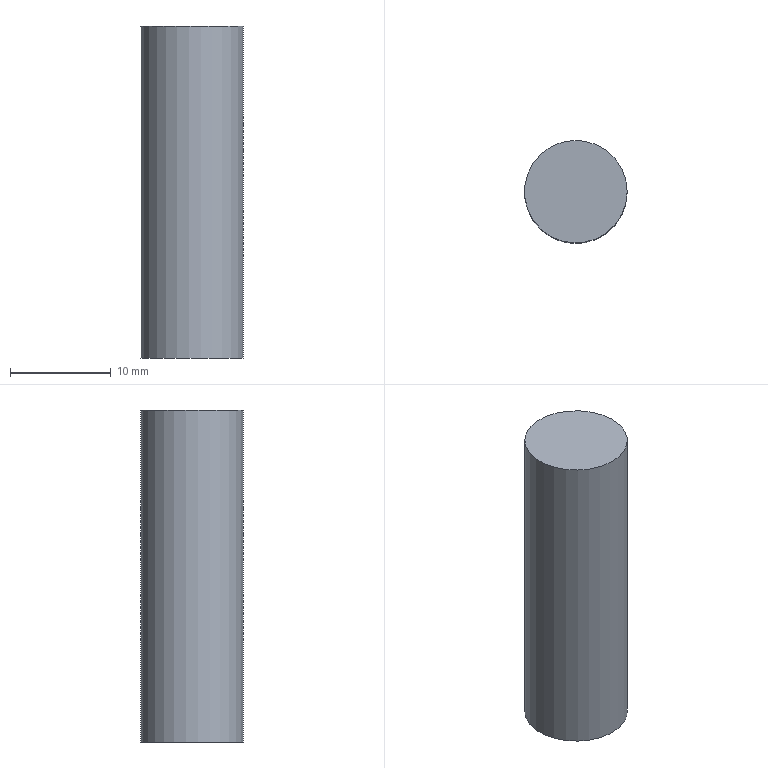Part | NX | features DATUM_CSYS 2, EXTRUDE 1, SKETCH 1 | 1 solid | 3 faces | box 10.2 x 10.2 x 33 mm | volume 2697 mm3 | plane 2 | cylinder 1 | commonest cylinder face diameters 10.2 x1
STEP:
#1=CARTESIAN_POINT('',(5.1,0.,-33.));
#2=VERTEX_POINT('',#1);
#3=CARTESIAN_POINT('',(0.,0.,-33.));
#4=DIRECTION('',(0.,0.,1.));
#5=DIRECTION('',(1.,0.,0.));
#6=AXIS2_PLACEMENT_3D('',#3,#4,#5);
#7=CIRCLE('',#6,5.1);
#8=EDGE_CURVE('',#2,#2,#7,.F.);
#9=ORIENTED_EDGE('',*,*,#8,.F.);
#10=EDGE_LOOP('',(#9));
#11=FACE_BOUND('',#10,.T.);
#12=CARTESIAN_POINT('',(5.1,0.,0.));
#13=VERTEX_POINT('',#12);
#14=CARTESIAN_POINT('',(0.,0.,0.));
#15=DIRECTION('',(0.,0.,1.));
#16=DIRECTION('',(1.,0.,0.));
#17=AXIS2_PLACEMENT_3D('',#14,#15,#16);
#18=CIRCLE('',#17,5.1);
#19=EDGE_CURVE('',#13,#13,#18,.F.);
#20=ORIENTED_EDGE('',*,*,#19,.T.);
#21=EDGE_LOOP('',(#20));
#22=FACE_BOUND('',#21,.T.);
#23=CARTESIAN_POINT('',(0.,0.,-33.));
#24=DIRECTION('',(0.,0.,1.));
#25=DIRECTION('',(1.,0.,0.));
#26=AXIS2_PLACEMENT_3D('',#23,#24,#25);
#27=CYLINDRICAL_SURFACE('',#26,5.1);
#28=ADVANCED_FACE('',(#11,#22),#27,.T.);
#29=ORIENTED_EDGE('',*,*,#8,.T.);
#30=EDGE_LOOP('',(#29));
#31=FACE_BOUND('',#30,.T.);
#32=CARTESIAN_POINT('',(0.,0.,-33.));
#33=DIRECTION('',(0.,0.,1.));
#34=DIRECTION('',(1.,0.,0.));
#35=AXIS2_PLACEMENT_3D('',#32,#33,#34);
#36=PLANE('',#35);
#37=ADVANCED_FACE('',(#31),#36,.F.);
#38=ORIENTED_EDGE('',*,*,#19,.F.);
#39=EDGE_LOOP('',(#38));
#40=FACE_BOUND('',#39,.T.);
#41=CARTESIAN_POINT('',(0.,0.,0.));
#42=DIRECTION('',(0.,0.,1.));
#43=DIRECTION('',(1.,0.,0.));
#44=AXIS2_PLACEMENT_3D('',#41,#42,#43);
#45=PLANE('',#44);
#46=ADVANCED_FACE('',(#40),#45,.T.);
#47=CLOSED_SHELL('',(#28,#37,#46));
#48=MANIFOLD_SOLID_BREP('',#47);
#49=(LENGTH_UNIT()NAMED_UNIT(*)SI_UNIT(.MILLI.,.METRE.));
#50=UNCERTAINTY_MEASURE_WITH_UNIT(LENGTH_MEASURE(0.00001),#49,'','');
#51=(NAMED_UNIT(*)PLANE_ANGLE_UNIT()SI_UNIT($,.RADIAN.));
#52=(NAMED_UNIT(*)SI_UNIT($,.STERADIAN.)SOLID_ANGLE_UNIT());
#53=(GEOMETRIC_REPRESENTATION_CONTEXT(3)GLOBAL_UNCERTAINTY_ASSIGNED_CONTEXT((#50))GLOBAL_UNIT_ASSIGNED_CONTEXT((#49,#51,#52))REPRESENTATION_CONTEXT('',''));
#54=ADVANCED_BREP_SHAPE_REPRESENTATION('',(#48),#53);